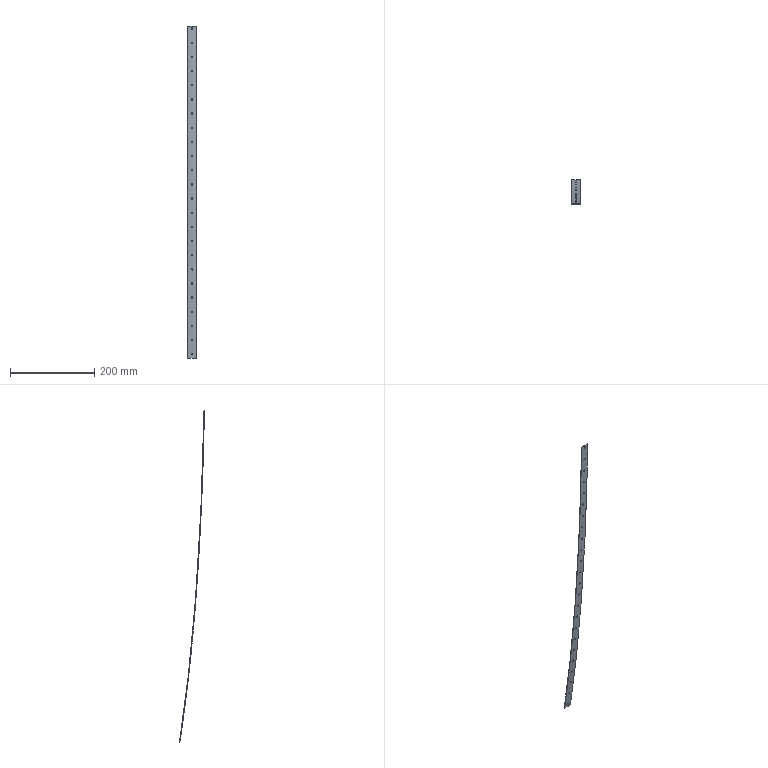Part | SolidWorks | features BaseBody 1 | 1 solid | 54 faces | box 20 x 59 x 788 mm | volume 15567 mm3 | cylinder 48 | plane 4 | spline 2 | commonest cylinder face diameters 3.2 x48